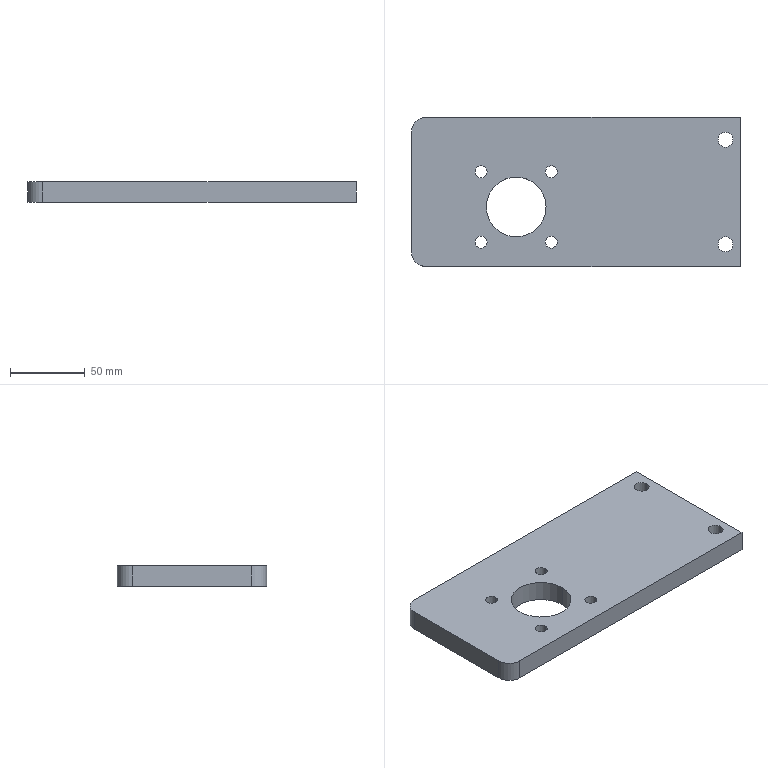Part | SolidWorks | features Fillet 1, FlatPattern 1, SMBaseFlange 1, SheetMetal 1 | 1 solid | 22 faces | box 220 x 100 x 14 mm | volume 284792 mm3 | cylinder 16 | plane 6 | commonest cylinder face diameters 8 x8 10 x4 20 x2 40 x2
STEP:
#1=CARTESIAN_POINT('',(89.5,-83.5,-14.));
#2=VERTEX_POINT('',#1);
#3=CARTESIAN_POINT('',(97.5,-83.5,-14.));
#4=VERTEX_POINT('',#3);
#5=CARTESIAN_POINT('',(93.5,-83.5,-14.));
#6=DIRECTION('',(0.,0.,1.));
#7=DIRECTION('',(1.,0.,0.));
#8=AXIS2_PLACEMENT_3D('',#5,#6,#7);
#9=CIRCLE('',#8,4.);
#10=EDGE_CURVE('',#2,#4,#9,.T.);
#11=ORIENTED_EDGE('',*,*,#10,.F.);
#12=CARTESIAN_POINT('',(89.5,-83.5,0.));
#13=VERTEX_POINT('',#12);
#14=CARTESIAN_POINT('',(89.5,-83.5,-14.));
#15=DIRECTION('',(0.,0.,1.));
#16=VECTOR('',#15,1000.);
#17=LINE('',#14,#16);
#18=EDGE_CURVE('',#2,#13,#17,.T.);
#19=ORIENTED_EDGE('',*,*,#18,.T.);
#20=CARTESIAN_POINT('',(97.5,-83.5,0.));
#21=VERTEX_POINT('',#20);
#22=CARTESIAN_POINT('',(93.5,-83.5,0.));
#23=DIRECTION('',(0.,0.,1.));
#24=DIRECTION('',(1.,0.,0.));
#25=AXIS2_PLACEMENT_3D('',#22,#23,#24);
#26=CIRCLE('',#25,4.);
#27=EDGE_CURVE('',#13,#21,#26,.T.);
#28=ORIENTED_EDGE('',*,*,#27,.T.);
#29=CARTESIAN_POINT('',(97.5,-83.5,-14.));
#30=DIRECTION('',(0.,0.,1.));
#31=VECTOR('',#30,1000.);
#32=LINE('',#29,#31);
#33=EDGE_CURVE('',#4,#21,#32,.T.);
#34=ORIENTED_EDGE('',*,*,#33,.F.);
#35=EDGE_LOOP('',(#11,#19,#28,#34));
#36=FACE_OUTER_BOUND('',#35,.T.);
#37=CARTESIAN_POINT('',(93.5,-83.5,-14.));
#38=DIRECTION('',(0.,0.,1.));
#39=DIRECTION('',(1.,0.,0.));
#40=AXIS2_PLACEMENT_3D('',#37,#38,#39);
#41=CYLINDRICAL_SURFACE('',#40,4.);
#42=ADVANCED_FACE('',(#36),#41,.F.);
#43=CARTESIAN_POINT('',(42.5,-83.5,-14.));
#44=VERTEX_POINT('',#43);
#45=CARTESIAN_POINT('',(50.5,-83.5,-14.));
#46=VERTEX_POINT('',#45);
#47=CARTESIAN_POINT('',(46.5,-83.5,-14.));
#48=DIRECTION('',(0.,0.,1.));
#49=DIRECTION('',(1.,0.,0.));
#50=AXIS2_PLACEMENT_3D('',#47,#48,#49);
#51=CIRCLE('',#50,4.);
#52=EDGE_CURVE('',#44,#46,#51,.T.);
#53=ORIENTED_EDGE('',*,*,#52,.F.);
#54=CARTESIAN_POINT('',(42.5,-83.5,0.));
#55=VERTEX_POINT('',#54);
#56=CARTESIAN_POINT('',(42.5,-83.5,-14.));
#57=DIRECTION('',(0.,0.,1.));
#58=VECTOR('',#57,1000.);
#59=LINE('',#56,#58);
#60=EDGE_CURVE('',#44,#55,#59,.T.);
#61=ORIENTED_EDGE('',*,*,#60,.T.);
#62=CARTESIAN_POINT('',(50.5,-83.5,0.));
#63=VERTEX_POINT('',#62);
#64=CARTESIAN_POINT('',(46.5,-83.5,0.));
#65=DIRECTION('',(0.,0.,1.));
#66=DIRECTION('',(1.,0.,0.));
#67=AXIS2_PLACEMENT_3D('',#64,#65,#66);
#68=CIRCLE('',#67,4.);
#69=EDGE_CURVE('',#55,#63,#68,.T.);
#70=ORIENTED_EDGE('',*,*,#69,.T.);
#71=CARTESIAN_POINT('',(50.5,-83.5,-14.));
#72=DIRECTION('',(0.,0.,1.));
#73=VECTOR('',#72,1000.);
#74=LINE('',#71,#73);
#75=EDGE_CURVE('',#46,#63,#74,.T.);
#76=ORIENTED_EDGE('',*,*,#75,.F.);
#77=EDGE_LOOP('',(#53,#61,#70,#76));
#78=FACE_OUTER_BOUND('',#77,.T.);
#79=CARTESIAN_POINT('',(46.5,-83.5,-14.));
#80=DIRECTION('',(0.,0.,1.));
#81=DIRECTION('',(1.,0.,0.));
#82=AXIS2_PLACEMENT_3D('',#79,#80,#81);
#83=CYLINDRICAL_SURFACE('',#82,4.);
#84=ADVANCED_FACE('',(#78),#83,.F.);
#85=CARTESIAN_POINT('',(89.5,-36.5,-14.));
#86=VERTEX_POINT('',#85);
#87=CARTESIAN_POINT('',(97.5,-36.5,-14.));
#88=VERTEX_POINT('',#87);
#89=CARTESIAN_POINT('',(93.5,-36.5,-14.));
#90=DIRECTION('',(0.,0.,1.));
#91=DIRECTION('',(1.,0.,0.));
#92=AXIS2_PLACEMENT_3D('',#89,#90,#91);
#93=CIRCLE('',#92,4.);
#94=EDGE_CURVE('',#86,#88,#93,.T.);
#95=ORIENTED_EDGE('',*,*,#94,.F.);
#96=CARTESIAN_POINT('',(89.5,-36.5,0.));
#97=VERTEX_POINT('',#96);
#98=CARTESIAN_POINT('',(89.5,-36.5,-14.));
#99=DIRECTION('',(0.,0.,1.));
#100=VECTOR('',#99,1000.);
#101=LINE('',#98,#100);
#102=EDGE_CURVE('',#86,#97,#101,.T.);
#103=ORIENTED_EDGE('',*,*,#102,.T.);
#104=CARTESIAN_POINT('',(97.5,-36.5,0.));
#105=VERTEX_POINT('',#104);
#106=CARTESIAN_POINT('',(93.5,-36.5,0.));
#107=DIRECTION('',(0.,0.,1.));
#108=DIRECTION('',(1.,0.,0.));
#109=AXIS2_PLACEMENT_3D('',#106,#107,#108);
#110=CIRCLE('',#109,4.);
#111=EDGE_CURVE('',#97,#105,#110,.T.);
#112=ORIENTED_EDGE('',*,*,#111,.T.);
#113=CARTESIAN_POINT('',(97.5,-36.5,-14.));
#114=DIRECTION('',(0.,0.,1.));
#115=VECTOR('',#114,1000.);
#116=LINE('',#113,#115);
#117=EDGE_CURVE('',#88,#105,#116,.T.);
#118=ORIENTED_EDGE('',*,*,#117,.F.);
#119=EDGE_LOOP('',(#95,#103,#112,#118));
#120=FACE_OUTER_BOUND('',#119,.T.);
#121=CARTESIAN_POINT('',(93.5,-36.5,-14.));
#122=DIRECTION('',(0.,0.,1.));
#123=DIRECTION('',(1.,0.,0.));
#124=AXIS2_PLACEMENT_3D('',#121,#122,#123);
#125=CYLINDRICAL_SURFACE('',#124,4.);
#126=ADVANCED_FACE('',(#120),#125,.F.);
#127=CARTESIAN_POINT('',(42.5,-36.5,-14.));
#128=VERTEX_POINT('',#127);
#129=CARTESIAN_POINT('',(50.5,-36.5,-14.));
#130=VERTEX_POINT('',#129);
#131=CARTESIAN_POINT('',(46.5,-36.5,-14.));
#132=DIRECTION('',(0.,0.,1.));
#133=DIRECTION('',(1.,0.,0.));
#134=AXIS2_PLACEMENT_3D('',#131,#132,#133);
#135=CIRCLE('',#134,4.);
#136=EDGE_CURVE('',#128,#130,#135,.T.);
#137=ORIENTED_EDGE('',*,*,#136,.F.);
#138=CARTESIAN_POINT('',(42.5,-36.5,0.));
#139=VERTEX_POINT('',#138);
#140=CARTESIAN_POINT('',(42.5,-36.5,-14.));
#141=DIRECTION('',(0.,0.,1.));
#142=VECTOR('',#141,1000.);
#143=LINE('',#140,#142);
#144=EDGE_CURVE('',#128,#139,#143,.T.);
#145=ORIENTED_EDGE('',*,*,#144,.T.);
#146=CARTESIAN_POINT('',(50.5,-36.5,0.));
#147=VERTEX_POINT('',#146);
#148=CARTESIAN_POINT('',(46.5,-36.5,0.));
#149=DIRECTION('',(0.,0.,1.));
#150=DIRECTION('',(1.,0.,0.));
#151=AXIS2_PLACEMENT_3D('',#148,#149,#150);
#152=CIRCLE('',#151,4.);
#153=EDGE_CURVE('',#139,#147,#152,.T.);
#154=ORIENTED_EDGE('',*,*,#153,.T.);
#155=CARTESIAN_POINT('',(50.5,-36.5,-14.));
#156=DIRECTION('',(0.,0.,1.));
#157=VECTOR('',#156,1000.);
#158=LINE('',#155,#157);
#159=EDGE_CURVE('',#130,#147,#158,.T.);
#160=ORIENTED_EDGE('',*,*,#159,.F.);
#161=EDGE_LOOP('',(#137,#145,#154,#160));
#162=FACE_OUTER_BOUND('',#161,.T.);
#163=CARTESIAN_POINT('',(46.5,-36.5,-14.));
#164=DIRECTION('',(0.,0.,1.));
#165=DIRECTION('',(1.,0.,0.));
#166=AXIS2_PLACEMENT_3D('',#163,#164,#165);
#167=CYLINDRICAL_SURFACE('',#166,4.);
#168=ADVANCED_FACE('',(#162),#167,.F.);
#169=CARTESIAN_POINT('',(50.,-60.,-14.));
#170=VERTEX_POINT('',#169);
#171=CARTESIAN_POINT('',(90.,-60.,-14.));
#172=VERTEX_POINT('',#171);
#173=CARTESIAN_POINT('',(70.,-60.,-14.));
#174=DIRECTION('',(0.,0.,1.));
#175=DIRECTION('',(1.,0.,0.));
#176=AXIS2_PLACEMENT_3D('',#173,#174,#175);
#177=CIRCLE('',#176,20.);
#178=EDGE_CURVE('',#170,#172,#177,.T.);
#179=ORIENTED_EDGE('',*,*,#178,.F.);
#180=CARTESIAN_POINT('',(50.,-60.,0.));
#181=VERTEX_POINT('',#180);
#182=CARTESIAN_POINT('',(50.,-60.,-14.));
#183=DIRECTION('',(0.,0.,1.));
#184=VECTOR('',#183,1000.);
#185=LINE('',#182,#184);
#186=EDGE_CURVE('',#170,#181,#185,.T.);
#187=ORIENTED_EDGE('',*,*,#186,.T.);
#188=CARTESIAN_POINT('',(90.,-60.,0.));
#189=VERTEX_POINT('',#188);
#190=CARTESIAN_POINT('',(70.,-60.,0.));
#191=DIRECTION('',(0.,0.,1.));
#192=DIRECTION('',(1.,0.,0.));
#193=AXIS2_PLACEMENT_3D('',#190,#191,#192);
#194=CIRCLE('',#193,20.);
#195=EDGE_CURVE('',#181,#189,#194,.T.);
#196=ORIENTED_EDGE('',*,*,#195,.T.);
#197=CARTESIAN_POINT('',(90.,-60.,-14.));
#198=DIRECTION('',(0.,0.,1.));
#199=VECTOR('',#198,1000.);
#200=LINE('',#197,#199);
#201=EDGE_CURVE('',#172,#189,#200,.T.);
#202=ORIENTED_EDGE('',*,*,#201,.F.);
#203=EDGE_LOOP('',(#179,#187,#196,#202));
#204=FACE_OUTER_BOUND('',#203,.T.);
#205=CARTESIAN_POINT('',(70.,-60.,-14.));
#206=DIRECTION('',(0.,0.,1.));
#207=DIRECTION('',(1.,0.,0.));
#208=AXIS2_PLACEMENT_3D('',#205,#206,#207);
#209=CYLINDRICAL_SURFACE('',#208,20.);
#210=ADVANCED_FACE('',(#204),#209,.F.);
#211=CARTESIAN_POINT('',(205.,-85.,-14.));
#212=VERTEX_POINT('',#211);
#213=CARTESIAN_POINT('',(215.,-85.,-14.));
#214=VERTEX_POINT('',#213);
#215=CARTESIAN_POINT('',(210.,-85.,-14.));
#216=DIRECTION('',(0.,0.,1.));
#217=DIRECTION('',(1.,0.,0.));
#218=AXIS2_PLACEMENT_3D('',#215,#216,#217);
#219=CIRCLE('',#218,5.);
#220=EDGE_CURVE('',#212,#214,#219,.T.);
#221=ORIENTED_EDGE('',*,*,#220,.F.);
#222=CARTESIAN_POINT('',(205.,-85.,0.));
#223=VERTEX_POINT('',#222);
#224=CARTESIAN_POINT('',(205.,-85.,-14.));
#225=DIRECTION('',(0.,0.,1.));
#226=VECTOR('',#225,1000.);
#227=LINE('',#224,#226);
#228=EDGE_CURVE('',#212,#223,#227,.T.);
#229=ORIENTED_EDGE('',*,*,#228,.T.);
#230=CARTESIAN_POINT('',(215.,-85.,0.));
#231=VERTEX_POINT('',#230);
#232=CARTESIAN_POINT('',(210.,-85.,0.));
#233=DIRECTION('',(0.,0.,1.));
#234=DIRECTION('',(1.,0.,0.));
#235=AXIS2_PLACEMENT_3D('',#232,#233,#234);
#236=CIRCLE('',#235,5.);
#237=EDGE_CURVE('',#223,#231,#236,.T.);
#238=ORIENTED_EDGE('',*,*,#237,.T.);
#239=CARTESIAN_POINT('',(215.,-85.,-14.));
#240=DIRECTION('',(0.,0.,1.));
#241=VECTOR('',#240,1000.);
#242=LINE('',#239,#241);
#243=EDGE_CURVE('',#214,#231,#242,.T.);
#244=ORIENTED_EDGE('',*,*,#243,.F.);
#245=EDGE_LOOP('',(#221,#229,#238,#244));
#246=FACE_OUTER_BOUND('',#245,.T.);
#247=CARTESIAN_POINT('',(210.,-85.,-14.));
#248=DIRECTION('',(0.,0.,1.));
#249=DIRECTION('',(1.,0.,0.));
#250=AXIS2_PLACEMENT_3D('',#247,#248,#249);
#251=CYLINDRICAL_SURFACE('',#250,5.);
#252=ADVANCED_FACE('',(#246),#251,.F.);
#253=CARTESIAN_POINT('',(205.,-15.,-14.));
#254=VERTEX_POINT('',#253);
#255=CARTESIAN_POINT('',(215.,-15.,-14.));
#256=VERTEX_POINT('',#255);
#257=CARTESIAN_POINT('',(210.,-15.,-14.));
#258=DIRECTION('',(0.,0.,1.));
#259=DIRECTION('',(1.,0.,0.));
#260=AXIS2_PLACEMENT_3D('',#257,#258,#259);
#261=CIRCLE('',#260,5.);
#262=EDGE_CURVE('',#254,#256,#261,.T.);
#263=ORIENTED_EDGE('',*,*,#262,.F.);
#264=CARTESIAN_POINT('',(205.,-15.,0.));
#265=VERTEX_POINT('',#264);
#266=CARTESIAN_POINT('',(205.,-15.,-14.));
#267=DIRECTION('',(0.,0.,1.));
#268=VECTOR('',#267,1000.);
#269=LINE('',#266,#268);
#270=EDGE_CURVE('',#254,#265,#269,.T.);
#271=ORIENTED_EDGE('',*,*,#270,.T.);
#272=CARTESIAN_POINT('',(215.,-15.,0.));
#273=VERTEX_POINT('',#272);
#274=CARTESIAN_POINT('',(210.,-15.,0.));
#275=DIRECTION('',(0.,0.,1.));
#276=DIRECTION('',(1.,0.,0.));
#277=AXIS2_PLACEMENT_3D('',#274,#275,#276);
#278=CIRCLE('',#277,5.);
#279=EDGE_CURVE('',#265,#273,#278,.T.);
#280=ORIENTED_EDGE('',*,*,#279,.T.);
#281=CARTESIAN_POINT('',(215.,-15.,-14.));
#282=DIRECTION('',(0.,0.,1.));
#283=VECTOR('',#282,1000.);
#284=LINE('',#281,#283);
#285=EDGE_CURVE('',#256,#273,#284,.T.);
#286=ORIENTED_EDGE('',*,*,#285,.F.);
#287=EDGE_LOOP('',(#263,#271,#280,#286));
#288=FACE_OUTER_BOUND('',#287,.T.);
#289=CARTESIAN_POINT('',(210.,-15.,-14.));
#290=DIRECTION('',(0.,0.,1.));
#291=DIRECTION('',(1.,0.,0.));
#292=AXIS2_PLACEMENT_3D('',#289,#290,#291);
#293=CYLINDRICAL_SURFACE('',#292,5.);
#294=ADVANCED_FACE('',(#288),#293,.F.);
#295=CARTESIAN_POINT('',(0.,-10.,0.));
#296=VERTEX_POINT('',#295);
#297=CARTESIAN_POINT('',(0.,-90.,0.));
#298=VERTEX_POINT('',#297);
#299=CARTESIAN_POINT('',(0.,0.,0.));
#300=DIRECTION('',(0.,-1.,0.));
#301=VECTOR('',#300,1000.);
#302=LINE('',#299,#301);
#303=EDGE_CURVE('',#296,#298,#302,.T.);
#304=ORIENTED_EDGE('',*,*,#303,.F.);
#305=CARTESIAN_POINT('',(0.,-10.,-14.));
#306=VERTEX_POINT('',#305);
#307=CARTESIAN_POINT('',(0.,-10.,-14.));
#308=DIRECTION('',(0.,0.,-1.));
#309=VECTOR('',#308,1000.);
#310=LINE('',#307,#309);
#311=EDGE_CURVE('',#296,#306,#310,.T.);
#312=ORIENTED_EDGE('',*,*,#311,.T.);
#313=CARTESIAN_POINT('',(0.,-90.,-14.));
#314=VERTEX_POINT('',#313);
#315=CARTESIAN_POINT('',(0.,0.,-14.));
#316=DIRECTION('',(0.,-1.,0.));
#317=VECTOR('',#316,1000.);
#318=LINE('',#315,#317);
#319=EDGE_CURVE('',#306,#314,#318,.T.);
#320=ORIENTED_EDGE('',*,*,#319,.T.);
#321=CARTESIAN_POINT('',(0.,-90.,-14.));
#322=DIRECTION('',(0.,0.,1.));
#323=VECTOR('',#322,1000.);
#324=LINE('',#321,#323);
#325=EDGE_CURVE('',#314,#298,#324,.T.);
#326=ORIENTED_EDGE('',*,*,#325,.T.);
#327=EDGE_LOOP('',(#304,#312,#320,#326));
#328=FACE_OUTER_BOUND('',#327,.T.);
#329=CARTESIAN_POINT('',(0.,0.,-14.));
#330=DIRECTION('',(-1.,0.,0.));
#331=DIRECTION('',(0.,0.,1.));
#332=AXIS2_PLACEMENT_3D('',#329,#330,#331);
#333=PLANE('',#332);
#334=ADVANCED_FACE('',(#328),#333,.T.);
#335=CARTESIAN_POINT('',(220.,0.,-14.));
#336=VERTEX_POINT('',#335);
#337=CARTESIAN_POINT('',(10.,0.,-14.));
#338=VERTEX_POINT('',#337);
#339=CARTESIAN_POINT('',(0.,0.,-14.));
#340=DIRECTION('',(-1.,0.,0.));
#341=VECTOR('',#340,1000.);
#342=LINE('',#339,#341);
#343=EDGE_CURVE('',#336,#338,#342,.T.);
#344=ORIENTED_EDGE('',*,*,#343,.T.);
#345=CARTESIAN_POINT('',(10.,0.,0.));
#346=VERTEX_POINT('',#345);
#347=CARTESIAN_POINT('',(10.,0.,-14.));
#348=DIRECTION('',(0.,0.,1.));
#349=VECTOR('',#348,1000.);
#350=LINE('',#347,#349);
#351=EDGE_CURVE('',#338,#346,#350,.T.);
#352=ORIENTED_EDGE('',*,*,#351,.T.);
#353=CARTESIAN_POINT('',(220.,0.,0.));
#354=VERTEX_POINT('',#353);
#355=CARTESIAN_POINT('',(0.,0.,0.));
#356=DIRECTION('',(-1.,0.,0.));
#357=VECTOR('',#356,1000.);
#358=LINE('',#355,#357);
#359=EDGE_CURVE('',#354,#346,#358,.T.);
#360=ORIENTED_EDGE('',*,*,#359,.F.);
#361=CARTESIAN_POINT('',(220.,0.,-14.));
#362=DIRECTION('',(0.,0.,1.));
#363=VECTOR('',#362,1000.);
#364=LINE('',#361,#363);
#365=EDGE_CURVE('',#336,#354,#364,.T.);
#366=ORIENTED_EDGE('',*,*,#365,.F.);
#367=EDGE_LOOP('',(#344,#352,#360,#366));
#368=FACE_OUTER_BOUND('',#367,.T.);
#369=CARTESIAN_POINT('',(0.,0.,-14.));
#370=DIRECTION('',(0.,1.,0.));
#371=DIRECTION('',(0.,0.,1.));
#372=AXIS2_PLACEMENT_3D('',#369,#370,#371);
#373=PLANE('',#372);
#374=ADVANCED_FACE('',(#368),#373,.T.);
#375=CARTESIAN_POINT('',(220.,-100.,0.));
#376=VERTEX_POINT('',#375);
#377=CARTESIAN_POINT('',(220.,0.,0.));
#378=DIRECTION('',(0.,1.,0.));
#379=VECTOR('',#378,1000.);
#380=LINE('',#377,#379);
#381=EDGE_CURVE('',#376,#354,#380,.T.);
#382=ORIENTED_EDGE('',*,*,#381,.F.);
#383=CARTESIAN_POINT('',(220.,-100.,-14.));
#384=VERTEX_POINT('',#383);
#385=CARTESIAN_POINT('',(220.,-100.,-14.));
#386=DIRECTION('',(0.,0.,1.));
#387=VECTOR('',#386,1000.);
#388=LINE('',#385,#387);
#389=EDGE_CURVE('',#384,#376,#388,.T.);
#390=ORIENTED_EDGE('',*,*,#389,.F.);
#391=CARTESIAN_POINT('',(220.,0.,-14.));
#392=DIRECTION('',(0.,1.,0.));
#393=VECTOR('',#392,1000.);
#394=LINE('',#391,#393);
#395=EDGE_CURVE('',#384,#336,#394,.T.);
#396=ORIENTED_EDGE('',*,*,#395,.T.);
#397=ORIENTED_EDGE('',*,*,#365,.T.);
#398=EDGE_LOOP('',(#382,#390,#396,#397));
#399=FACE_OUTER_BOUND('',#398,.T.);
#400=CARTESIAN_POINT('',(220.,0.,-14.));
#401=DIRECTION('',(1.,0.,0.));
#402=DIRECTION('',(0.,0.,-1.));
#403=AXIS2_PLACEMENT_3D('',#400,#401,#402);
#404=PLANE('',#403);
#405=ADVANCED_FACE('',(#399),#404,.T.);
#406=CARTESIAN_POINT('',(10.,-100.,0.));
#407=VERTEX_POINT('',#406);
#408=CARTESIAN_POINT('',(0.,-100.,0.));
#409=DIRECTION('',(1.,0.,0.));
#410=VECTOR('',#409,1000.);
#411=LINE('',#408,#410);
#412=EDGE_CURVE('',#407,#376,#411,.T.);
#413=ORIENTED_EDGE('',*,*,#412,.F.);
#414=CARTESIAN_POINT('',(10.,-100.,-14.));
#415=VERTEX_POINT('',#414);
#416=CARTESIAN_POINT('',(10.,-100.,-14.));
#417=DIRECTION('',(0.,0.,-1.));
#418=VECTOR('',#417,1000.);
#419=LINE('',#416,#418);
#420=EDGE_CURVE('',#407,#415,#419,.T.);
#421=ORIENTED_EDGE('',*,*,#420,.T.);
#422=CARTESIAN_POINT('',(0.,-100.,-14.));
#423=DIRECTION('',(1.,0.,0.));
#424=VECTOR('',#423,1000.);
#425=LINE('',#422,#424);
#426=EDGE_CURVE('',#415,#384,#425,.T.);
#427=ORIENTED_EDGE('',*,*,#426,.T.);
#428=ORIENTED_EDGE('',*,*,#389,.T.);
#429=EDGE_LOOP('',(#413,#421,#427,#428));
#430=FACE_OUTER_BOUND('',#429,.T.);
#431=CARTESIAN_POINT('',(0.,-100.,-14.));
#432=DIRECTION('',(0.,-1.,0.));
#433=DIRECTION('',(0.,0.,-1.));
#434=AXIS2_PLACEMENT_3D('',#431,#432,#433);
#435=PLANE('',#434);
#436=ADVANCED_FACE('',(#430),#435,.T.);
#437=CARTESIAN_POINT('',(93.5,-83.5,-14.));
#438=DIRECTION('',(0.,0.,1.));
#439=DIRECTION('',(1.,0.,0.));
#440=AXIS2_PLACEMENT_3D('',#437,#438,#439);
#441=CIRCLE('',#440,4.);
#442=EDGE_CURVE('',#4,#2,#441,.T.);
#443=ORIENTED_EDGE('',*,*,#442,.T.);
#444=ORIENTED_EDGE('',*,*,#10,.T.);
#445=EDGE_LOOP('',(#443,#444));
#446=FACE_BOUND('',#445,.T.);
#447=CARTESIAN_POINT('',(46.5,-83.5,-14.));
#448=DIRECTION('',(0.,0.,1.));
#449=DIRECTION('',(1.,0.,0.));
#450=AXIS2_PLACEMENT_3D('',#447,#448,#449);
#451=CIRCLE('',#450,4.);
#452=EDGE_CURVE('',#46,#44,#451,.T.);
#453=ORIENTED_EDGE('',*,*,#452,.T.);
#454=ORIENTED_EDGE('',*,*,#52,.T.);
#455=EDGE_LOOP('',(#453,#454));
#456=FACE_BOUND('',#455,.T.);
#457=CARTESIAN_POINT('',(93.5,-36.5,-14.));
#458=DIRECTION('',(0.,0.,1.));
#459=DIRECTION('',(1.,0.,0.));
#460=AXIS2_PLACEMENT_3D('',#457,#458,#459);
#461=CIRCLE('',#460,4.);
#462=EDGE_CURVE('',#88,#86,#461,.T.);
#463=ORIENTED_EDGE('',*,*,#462,.T.);
#464=ORIENTED_EDGE('',*,*,#94,.T.);
#465=EDGE_LOOP('',(#463,#464));
#466=FACE_BOUND('',#465,.T.);
#467=CARTESIAN_POINT('',(46.5,-36.5,-14.));
#468=DIRECTION('',(0.,0.,1.));
#469=DIRECTION('',(1.,0.,0.));
#470=AXIS2_PLACEMENT_3D('',#467,#468,#469);
#471=CIRCLE('',#470,4.);
#472=EDGE_CURVE('',#130,#128,#471,.T.);
#473=ORIENTED_EDGE('',*,*,#472,.T.);
#474=ORIENTED_EDGE('',*,*,#136,.T.);
#475=EDGE_LOOP('',(#473,#474));
#476=FACE_BOUND('',#475,.T.);
#477=CARTESIAN_POINT('',(70.,-60.,-14.));
#478=DIRECTION('',(0.,0.,1.));
#479=DIRECTION('',(1.,0.,0.));
#480=AXIS2_PLACEMENT_3D('',#477,#478,#479);
#481=CIRCLE('',#480,20.);
#482=EDGE_CURVE('',#172,#170,#481,.T.);
#483=ORIENTED_EDGE('',*,*,#482,.T.);
#484=ORIENTED_EDGE('',*,*,#178,.T.);
#485=EDGE_LOOP('',(#483,#484));
#486=FACE_BOUND('',#485,.T.);
#487=CARTESIAN_POINT('',(210.,-85.,-14.));
#488=DIRECTION('',(0.,0.,1.));
#489=DIRECTION('',(1.,0.,0.));
#490=AXIS2_PLACEMENT_3D('',#487,#488,#489);
#491=CIRCLE('',#490,5.);
#492=EDGE_CURVE('',#214,#212,#491,.T.);
#493=ORIENTED_EDGE('',*,*,#492,.T.);
#494=ORIENTED_EDGE('',*,*,#220,.T.);
#495=EDGE_LOOP('',(#493,#494));
#496=FACE_BOUND('',#495,.T.);
#497=CARTESIAN_POINT('',(210.,-15.,-14.));
#498=DIRECTION('',(0.,0.,1.));
#499=DIRECTION('',(1.,0.,0.));
#500=AXIS2_PLACEMENT_3D('',#497,#498,#499);
#501=CIRCLE('',#500,5.);
#502=EDGE_CURVE('',#256,#254,#501,.T.);
#503=ORIENTED_EDGE('',*,*,#502,.T.);
#504=ORIENTED_EDGE('',*,*,#262,.T.);
#505=EDGE_LOOP('',(#503,#504));
#506=FACE_BOUND('',#505,.T.);
#507=ORIENTED_EDGE('',*,*,#319,.F.);
#508=CARTESIAN_POINT('',(10.,-10.,-14.));
#509=DIRECTION('',(0.,0.,-1.));
#510=DIRECTION('',(1.,0.,0.));
#511=AXIS2_PLACEMENT_3D('',#508,#509,#510);
#512=CIRCLE('',#511,10.);
#513=EDGE_CURVE('',#306,#338,#512,.T.);
#514=ORIENTED_EDGE('',*,*,#513,.T.);
#515=ORIENTED_EDGE('',*,*,#343,.F.);
#516=ORIENTED_EDGE('',*,*,#395,.F.);
#517=ORIENTED_EDGE('',*,*,#426,.F.);
#518=CARTESIAN_POINT('',(10.,-90.,-14.));
#519=DIRECTION('',(0.,0.,-1.));
#520=DIRECTION('',(1.,0.,0.));
#521=AXIS2_PLACEMENT_3D('',#518,#519,#520);
#522=CIRCLE('',#521,10.);
#523=EDGE_CURVE('',#415,#314,#522,.T.);
#524=ORIENTED_EDGE('',*,*,#523,.T.);
#525=EDGE_LOOP('',(#507,#514,#515,#516,#517,#524));
#526=FACE_OUTER_BOUND('',#525,.T.);
#527=CARTESIAN_POINT('',(0.,0.,-14.));
#528=DIRECTION('',(0.,0.,1.));
#529=DIRECTION('',(1.,0.,0.));
#530=AXIS2_PLACEMENT_3D('',#527,#528,#529);
#531=PLANE('',#530);
#532=ADVANCED_FACE('',(#446,#456,#466,#476,#486,#496,#506,#526),#531,.F.);
#533=CARTESIAN_POINT('',(93.5,-83.5,0.));
#534=DIRECTION('',(0.,0.,1.));
#535=DIRECTION('',(1.,0.,0.));
#536=AXIS2_PLACEMENT_3D('',#533,#534,#535);
#537=CIRCLE('',#536,4.);
#538=EDGE_CURVE('',#21,#13,#537,.T.);
#539=ORIENTED_EDGE('',*,*,#538,.F.);
#540=ORIENTED_EDGE('',*,*,#27,.F.);
#541=EDGE_LOOP('',(#539,#540));
#542=FACE_BOUND('',#541,.T.);
#543=CARTESIAN_POINT('',(46.5,-83.5,0.));
#544=DIRECTION('',(0.,0.,1.));
#545=DIRECTION('',(1.,0.,0.));
#546=AXIS2_PLACEMENT_3D('',#543,#544,#545);
#547=CIRCLE('',#546,4.);
#548=EDGE_CURVE('',#63,#55,#547,.T.);
#549=ORIENTED_EDGE('',*,*,#548,.F.);
#550=ORIENTED_EDGE('',*,*,#69,.F.);
#551=EDGE_LOOP('',(#549,#550));
#552=FACE_BOUND('',#551,.T.);
#553=CARTESIAN_POINT('',(93.5,-36.5,0.));
#554=DIRECTION('',(0.,0.,1.));
#555=DIRECTION('',(1.,0.,0.));
#556=AXIS2_PLACEMENT_3D('',#553,#554,#555);
#557=CIRCLE('',#556,4.);
#558=EDGE_CURVE('',#105,#97,#557,.T.);
#559=ORIENTED_EDGE('',*,*,#558,.F.);
#560=ORIENTED_EDGE('',*,*,#111,.F.);
#561=EDGE_LOOP('',(#559,#560));
#562=FACE_BOUND('',#561,.T.);
#563=CARTESIAN_POINT('',(46.5,-36.5,0.));
#564=DIRECTION('',(0.,0.,1.));
#565=DIRECTION('',(1.,0.,0.));
#566=AXIS2_PLACEMENT_3D('',#563,#564,#565);
#567=CIRCLE('',#566,4.);
#568=EDGE_CURVE('',#147,#139,#567,.T.);
#569=ORIENTED_EDGE('',*,*,#568,.F.);
#570=ORIENTED_EDGE('',*,*,#153,.F.);
#571=EDGE_LOOP('',(#569,#570));
#572=FACE_BOUND('',#571,.T.);
#573=CARTESIAN_POINT('',(70.,-60.,0.));
#574=DIRECTION('',(0.,0.,1.));
#575=DIRECTION('',(1.,0.,0.));
#576=AXIS2_PLACEMENT_3D('',#573,#574,#575);
#577=CIRCLE('',#576,20.);
#578=EDGE_CURVE('',#189,#181,#577,.T.);
#579=ORIENTED_EDGE('',*,*,#578,.F.);
#580=ORIENTED_EDGE('',*,*,#195,.F.);
#581=EDGE_LOOP('',(#579,#580));
#582=FACE_BOUND('',#581,.T.);
#583=CARTESIAN_POINT('',(210.,-85.,0.));
#584=DIRECTION('',(0.,0.,1.));
#585=DIRECTION('',(1.,0.,0.));
#586=AXIS2_PLACEMENT_3D('',#583,#584,#585);
#587=CIRCLE('',#586,5.);
#588=EDGE_CURVE('',#231,#223,#587,.T.);
#589=ORIENTED_EDGE('',*,*,#588,.F.);
#590=ORIENTED_EDGE('',*,*,#237,.F.);
#591=EDGE_LOOP('',(#589,#590));
#592=FACE_BOUND('',#591,.T.);
#593=CARTESIAN_POINT('',(210.,-15.,0.));
#594=DIRECTION('',(0.,0.,1.));
#595=DIRECTION('',(1.,0.,0.));
#596=AXIS2_PLACEMENT_3D('',#593,#594,#595);
#597=CIRCLE('',#596,5.);
#598=EDGE_CURVE('',#273,#265,#597,.T.);
#599=ORIENTED_EDGE('',*,*,#598,.F.);
#600=ORIENTED_EDGE('',*,*,#279,.F.);
#601=EDGE_LOOP('',(#599,#600));
#602=FACE_BOUND('',#601,.T.);
#603=ORIENTED_EDGE('',*,*,#359,.T.);
#604=CARTESIAN_POINT('',(10.,-10.,0.));
#605=DIRECTION('',(0.,0.,1.));
#606=DIRECTION('',(1.,0.,0.));
#607=AXIS2_PLACEMENT_3D('',#604,#605,#606);
#608=CIRCLE('',#607,10.);
#609=EDGE_CURVE('',#346,#296,#608,.T.);
#610=ORIENTED_EDGE('',*,*,#609,.T.);
#611=ORIENTED_EDGE('',*,*,#303,.T.);
#612=CARTESIAN_POINT('',(10.,-90.,0.));
#613=DIRECTION('',(0.,0.,1.));
#614=DIRECTION('',(1.,0.,0.));
#615=AXIS2_PLACEMENT_3D('',#612,#613,#614);
#616=CIRCLE('',#615,10.);
#617=EDGE_CURVE('',#298,#407,#616,.T.);
#618=ORIENTED_EDGE('',*,*,#617,.T.);
#619=ORIENTED_EDGE('',*,*,#412,.T.);
#620=ORIENTED_EDGE('',*,*,#381,.T.);
#621=EDGE_LOOP('',(#603,#610,#611,#618,#619,#620));
#622=FACE_OUTER_BOUND('',#621,.T.);
#623=CARTESIAN_POINT('',(0.,0.,0.));
#624=DIRECTION('',(0.,0.,1.));
#625=DIRECTION('',(1.,0.,0.));
#626=AXIS2_PLACEMENT_3D('',#623,#624,#625);
#627=PLANE('',#626);
#628=ADVANCED_FACE('',(#542,#552,#562,#572,#582,#592,#602,#622),#627,.T.);
#629=ORIENTED_EDGE('',*,*,#270,.F.);
#630=ORIENTED_EDGE('',*,*,#502,.F.);
#631=ORIENTED_EDGE('',*,*,#285,.T.);
#632=ORIENTED_EDGE('',*,*,#598,.T.);
#633=EDGE_LOOP('',(#629,#630,#631,#632));
#634=FACE_OUTER_BOUND('',#633,.T.);
#635=CARTESIAN_POINT('',(210.,-15.,-14.));
#636=DIRECTION('',(0.,0.,1.));
#637=DIRECTION('',(1.,0.,0.));
#638=AXIS2_PLACEMENT_3D('',#635,#636,#637);
#639=CYLINDRICAL_SURFACE('',#638,5.);
#640=ADVANCED_FACE('',(#634),#639,.F.);
#641=ORIENTED_EDGE('',*,*,#228,.F.);
#642=ORIENTED_EDGE('',*,*,#492,.F.);
#643=ORIENTED_EDGE('',*,*,#243,.T.);
#644=ORIENTED_EDGE('',*,*,#588,.T.);
#645=EDGE_LOOP('',(#641,#642,#643,#644));
#646=FACE_OUTER_BOUND('',#645,.T.);
#647=CARTESIAN_POINT('',(210.,-85.,-14.));
#648=DIRECTION('',(0.,0.,1.));
#649=DIRECTION('',(1.,0.,0.));
#650=AXIS2_PLACEMENT_3D('',#647,#648,#649);
#651=CYLINDRICAL_SURFACE('',#650,5.);
#652=ADVANCED_FACE('',(#646),#651,.F.);
#653=ORIENTED_EDGE('',*,*,#186,.F.);
#654=ORIENTED_EDGE('',*,*,#482,.F.);
#655=ORIENTED_EDGE('',*,*,#201,.T.);
#656=ORIENTED_EDGE('',*,*,#578,.T.);
#657=EDGE_LOOP('',(#653,#654,#655,#656));
#658=FACE_OUTER_BOUND('',#657,.T.);
#659=CARTESIAN_POINT('',(70.,-60.,-14.));
#660=DIRECTION('',(0.,0.,1.));
#661=DIRECTION('',(1.,0.,0.));
#662=AXIS2_PLACEMENT_3D('',#659,#660,#661);
#663=CYLINDRICAL_SURFACE('',#662,20.);
#664=ADVANCED_FACE('',(#658),#663,.F.);
#665=ORIENTED_EDGE('',*,*,#144,.F.);
#666=ORIENTED_EDGE('',*,*,#472,.F.);
#667=ORIENTED_EDGE('',*,*,#159,.T.);
#668=ORIENTED_EDGE('',*,*,#568,.T.);
#669=EDGE_LOOP('',(#665,#666,#667,#668));
#670=FACE_OUTER_BOUND('',#669,.T.);
#671=CARTESIAN_POINT('',(46.5,-36.5,-14.));
#672=DIRECTION('',(0.,0.,1.));
#673=DIRECTION('',(1.,0.,0.));
#674=AXIS2_PLACEMENT_3D('',#671,#672,#673);
#675=CYLINDRICAL_SURFACE('',#674,4.);
#676=ADVANCED_FACE('',(#670),#675,.F.);
#677=ORIENTED_EDGE('',*,*,#102,.F.);
#678=ORIENTED_EDGE('',*,*,#462,.F.);
#679=ORIENTED_EDGE('',*,*,#117,.T.);
#680=ORIENTED_EDGE('',*,*,#558,.T.);
#681=EDGE_LOOP('',(#677,#678,#679,#680));
#682=FACE_OUTER_BOUND('',#681,.T.);
#683=CARTESIAN_POINT('',(93.5,-36.5,-14.));
#684=DIRECTION('',(0.,0.,1.));
#685=DIRECTION('',(1.,0.,0.));
#686=AXIS2_PLACEMENT_3D('',#683,#684,#685);
#687=CYLINDRICAL_SURFACE('',#686,4.);
#688=ADVANCED_FACE('',(#682),#687,.F.);
#689=ORIENTED_EDGE('',*,*,#60,.F.);
#690=ORIENTED_EDGE('',*,*,#452,.F.);
#691=ORIENTED_EDGE('',*,*,#75,.T.);
#692=ORIENTED_EDGE('',*,*,#548,.T.);
#693=EDGE_LOOP('',(#689,#690,#691,#692));
#694=FACE_OUTER_BOUND('',#693,.T.);
#695=CARTESIAN_POINT('',(46.5,-83.5,-14.));
#696=DIRECTION('',(0.,0.,1.));
#697=DIRECTION('',(1.,0.,0.));
#698=AXIS2_PLACEMENT_3D('',#695,#696,#697);
#699=CYLINDRICAL_SURFACE('',#698,4.);
#700=ADVANCED_FACE('',(#694),#699,.F.);
#701=ORIENTED_EDGE('',*,*,#18,.F.);
#702=ORIENTED_EDGE('',*,*,#442,.F.);
#703=ORIENTED_EDGE('',*,*,#33,.T.);
#704=ORIENTED_EDGE('',*,*,#538,.T.);
#705=EDGE_LOOP('',(#701,#702,#703,#704));
#706=FACE_OUTER_BOUND('',#705,.T.);
#707=CARTESIAN_POINT('',(93.5,-83.5,-14.));
#708=DIRECTION('',(0.,0.,1.));
#709=DIRECTION('',(1.,0.,0.));
#710=AXIS2_PLACEMENT_3D('',#707,#708,#709);
#711=CYLINDRICAL_SURFACE('',#710,4.);
#712=ADVANCED_FACE('',(#706),#711,.F.);
#713=ORIENTED_EDGE('',*,*,#513,.F.);
#714=ORIENTED_EDGE('',*,*,#311,.F.);
#715=ORIENTED_EDGE('',*,*,#609,.F.);
#716=ORIENTED_EDGE('',*,*,#351,.F.);
#717=EDGE_LOOP('',(#713,#714,#715,#716));
#718=FACE_OUTER_BOUND('',#717,.T.);
#719=CARTESIAN_POINT('',(10.,-10.,-14.));
#720=DIRECTION('',(0.,0.,1.));
#721=DIRECTION('',(1.,0.,0.));
#722=AXIS2_PLACEMENT_3D('',#719,#720,#721);
#723=CYLINDRICAL_SURFACE('',#722,10.);
#724=ADVANCED_FACE('',(#718),#723,.T.);
#725=ORIENTED_EDGE('',*,*,#523,.F.);
#726=ORIENTED_EDGE('',*,*,#420,.F.);
#727=ORIENTED_EDGE('',*,*,#617,.F.);
#728=ORIENTED_EDGE('',*,*,#325,.F.);
#729=EDGE_LOOP('',(#725,#726,#727,#728));
#730=FACE_OUTER_BOUND('',#729,.T.);
#731=CARTESIAN_POINT('',(10.,-90.,-14.));
#732=DIRECTION('',(0.,0.,1.));
#733=DIRECTION('',(1.,0.,0.));
#734=AXIS2_PLACEMENT_3D('',#731,#732,#733);
#735=CYLINDRICAL_SURFACE('',#734,10.);
#736=ADVANCED_FACE('',(#730),#735,.T.);
#737=CLOSED_SHELL('',(#42,#84,#126,#168,#210,#252,#294,#334,#374,#405,#436,#532,#628,#640,#652,#664,#676,#688,#700,#712,#724,#736));
#738=MANIFOLD_SOLID_BREP('',#737);
#739=CARTESIAN_POINT('',(0.,0.,0.));
#740=DIRECTION('',(0.,0.,1.));
#741=DIRECTION('',(1.,0.,0.));
#742=AXIS2_PLACEMENT_3D('',#739,#740,#741);
#743=(LENGTH_UNIT()NAMED_UNIT(*)SI_UNIT(.MILLI.,.METRE.));
#744=UNCERTAINTY_MEASURE_WITH_UNIT(LENGTH_MEASURE(0.00001),#743,'','');
#745=(NAMED_UNIT(*)PLANE_ANGLE_UNIT()SI_UNIT($,.RADIAN.));
#746=(NAMED_UNIT(*)SI_UNIT($,.STERADIAN.)SOLID_ANGLE_UNIT());
#747=(GEOMETRIC_REPRESENTATION_CONTEXT(3)GLOBAL_UNCERTAINTY_ASSIGNED_CONTEXT((#744))GLOBAL_UNIT_ASSIGNED_CONTEXT((#743,#745,#746))REPRESENTATION_CONTEXT('',''));
#748=ADVANCED_BREP_SHAPE_REPRESENTATION('',(#738,#742),#747);